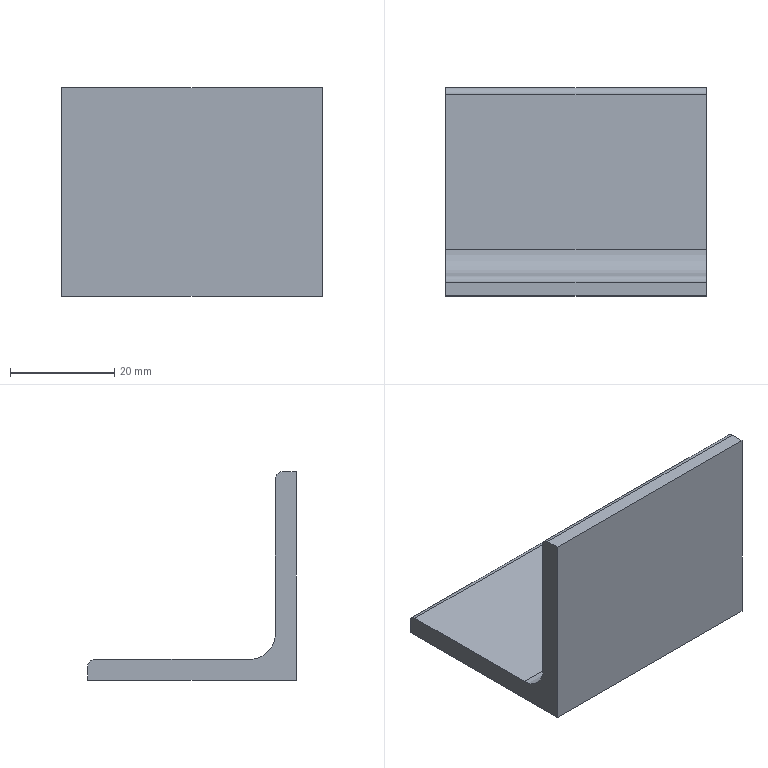Part | SolidWorks | features Extrusion 1 | 1 solid | 11 faces | box 50 x 40 x 40 mm | volume 15430 mm3 | plane 8 | cylinder 3 | commonest cylinder face diameters 2.667 x2 10 x1
STEP:
#1=CARTESIAN_POINT('',(0.,2.667,40.));
#2=VERTEX_POINT('',#1);
#3=CARTESIAN_POINT('',(0.,0.,40.));
#4=VERTEX_POINT('',#3);
#5=CARTESIAN_POINT('',(0.,0.,40.));
#6=DIRECTION('',(0.,-1.,0.));
#7=VECTOR('',#6,1000.);
#8=LINE('',#5,#7);
#9=EDGE_CURVE('',#2,#4,#8,.T.);
#10=ORIENTED_EDGE('',*,*,#9,.T.);
#11=CARTESIAN_POINT('',(50.,0.,40.));
#12=VERTEX_POINT('',#11);
#13=CARTESIAN_POINT('',(50.,0.,40.));
#14=DIRECTION('',(-1.,0.,0.));
#15=VECTOR('',#14,1000.);
#16=LINE('',#13,#15);
#17=EDGE_CURVE('',#12,#4,#16,.T.);
#18=ORIENTED_EDGE('',*,*,#17,.F.);
#19=CARTESIAN_POINT('',(50.,2.667,40.));
#20=VERTEX_POINT('',#19);
#21=CARTESIAN_POINT('',(50.,0.,40.));
#22=DIRECTION('',(0.,-1.,0.));
#23=VECTOR('',#22,1000.);
#24=LINE('',#21,#23);
#25=EDGE_CURVE('',#20,#12,#24,.T.);
#26=ORIENTED_EDGE('',*,*,#25,.F.);
#27=CARTESIAN_POINT('',(50.,2.667,40.));
#28=DIRECTION('',(-1.,0.,0.));
#29=VECTOR('',#28,1000.);
#30=LINE('',#27,#29);
#31=EDGE_CURVE('',#20,#2,#30,.T.);
#32=ORIENTED_EDGE('',*,*,#31,.T.);
#33=EDGE_LOOP('',(#10,#18,#26,#32));
#34=FACE_OUTER_BOUND('',#33,.T.);
#35=CARTESIAN_POINT('',(50.,0.,40.));
#36=DIRECTION('',(0.,0.,-1.));
#37=DIRECTION('',(0.,1.,0.));
#38=AXIS2_PLACEMENT_3D('',#35,#36,#37);
#39=PLANE('',#38);
#40=ADVANCED_FACE('',(#34),#39,.F.);
#41=CARTESIAN_POINT('',(0.,0.,0.));
#42=VERTEX_POINT('',#41);
#43=CARTESIAN_POINT('',(0.,0.,40.));
#44=DIRECTION('',(0.,0.,-1.));
#45=VECTOR('',#44,1000.);
#46=LINE('',#43,#45);
#47=EDGE_CURVE('',#4,#42,#46,.T.);
#48=ORIENTED_EDGE('',*,*,#47,.T.);
#49=CARTESIAN_POINT('',(50.,0.,0.));
#50=VERTEX_POINT('',#49);
#51=CARTESIAN_POINT('',(50.,0.,0.));
#52=DIRECTION('',(-1.,0.,0.));
#53=VECTOR('',#52,1000.);
#54=LINE('',#51,#53);
#55=EDGE_CURVE('',#50,#42,#54,.T.);
#56=ORIENTED_EDGE('',*,*,#55,.F.);
#57=CARTESIAN_POINT('',(50.,0.,40.));
#58=DIRECTION('',(0.,0.,-1.));
#59=VECTOR('',#58,1000.);
#60=LINE('',#57,#59);
#61=EDGE_CURVE('',#12,#50,#60,.T.);
#62=ORIENTED_EDGE('',*,*,#61,.F.);
#63=ORIENTED_EDGE('',*,*,#17,.T.);
#64=EDGE_LOOP('',(#48,#56,#62,#63));
#65=FACE_OUTER_BOUND('',#64,.T.);
#66=CARTESIAN_POINT('',(50.,0.,40.));
#67=DIRECTION('',(0.,1.,0.));
#68=DIRECTION('',(0.,0.,1.));
#69=AXIS2_PLACEMENT_3D('',#66,#67,#68);
#70=PLANE('',#69);
#71=ADVANCED_FACE('',(#65),#70,.F.);
#72=CARTESIAN_POINT('',(0.,40.,0.));
#73=VERTEX_POINT('',#72);
#74=CARTESIAN_POINT('',(0.,0.,0.));
#75=DIRECTION('',(0.,1.,0.));
#76=VECTOR('',#75,1000.);
#77=LINE('',#74,#76);
#78=EDGE_CURVE('',#42,#73,#77,.T.);
#79=ORIENTED_EDGE('',*,*,#78,.T.);
#80=CARTESIAN_POINT('',(50.,40.,0.));
#81=VERTEX_POINT('',#80);
#82=CARTESIAN_POINT('',(50.,40.,0.));
#83=DIRECTION('',(-1.,0.,0.));
#84=VECTOR('',#83,1000.);
#85=LINE('',#82,#84);
#86=EDGE_CURVE('',#81,#73,#85,.T.);
#87=ORIENTED_EDGE('',*,*,#86,.F.);
#88=CARTESIAN_POINT('',(50.,0.,0.));
#89=DIRECTION('',(0.,1.,0.));
#90=VECTOR('',#89,1000.);
#91=LINE('',#88,#90);
#92=EDGE_CURVE('',#50,#81,#91,.T.);
#93=ORIENTED_EDGE('',*,*,#92,.F.);
#94=ORIENTED_EDGE('',*,*,#55,.T.);
#95=EDGE_LOOP('',(#79,#87,#93,#94));
#96=FACE_OUTER_BOUND('',#95,.T.);
#97=CARTESIAN_POINT('',(50.,0.,0.));
#98=DIRECTION('',(0.,0.,1.));
#99=DIRECTION('',(1.,0.,0.));
#100=AXIS2_PLACEMENT_3D('',#97,#98,#99);
#101=PLANE('',#100);
#102=ADVANCED_FACE('',(#96),#101,.F.);
#103=CARTESIAN_POINT('',(0.,40.,2.667));
#104=VERTEX_POINT('',#103);
#105=CARTESIAN_POINT('',(0.,40.,0.));
#106=DIRECTION('',(0.,0.,1.));
#107=VECTOR('',#106,1000.);
#108=LINE('',#105,#107);
#109=EDGE_CURVE('',#73,#104,#108,.T.);
#110=ORIENTED_EDGE('',*,*,#109,.T.);
#111=CARTESIAN_POINT('',(50.,40.,2.667));
#112=VERTEX_POINT('',#111);
#113=CARTESIAN_POINT('',(50.,40.,2.667));
#114=DIRECTION('',(-1.,0.,0.));
#115=VECTOR('',#114,1000.);
#116=LINE('',#113,#115);
#117=EDGE_CURVE('',#112,#104,#116,.T.);
#118=ORIENTED_EDGE('',*,*,#117,.F.);
#119=CARTESIAN_POINT('',(50.,40.,0.));
#120=DIRECTION('',(0.,0.,1.));
#121=VECTOR('',#120,1000.);
#122=LINE('',#119,#121);
#123=EDGE_CURVE('',#81,#112,#122,.T.);
#124=ORIENTED_EDGE('',*,*,#123,.F.);
#125=ORIENTED_EDGE('',*,*,#86,.T.);
#126=EDGE_LOOP('',(#110,#118,#124,#125));
#127=FACE_OUTER_BOUND('',#126,.T.);
#128=CARTESIAN_POINT('',(50.,40.,0.));
#129=DIRECTION('',(0.,-1.,0.));
#130=DIRECTION('',(0.,0.,-1.));
#131=AXIS2_PLACEMENT_3D('',#128,#129,#130);
#132=PLANE('',#131);
#133=ADVANCED_FACE('',(#127),#132,.F.);
#134=CARTESIAN_POINT('',(0.,38.667,4.));
#135=VERTEX_POINT('',#134);
#136=CARTESIAN_POINT('',(0.,38.667,2.667));
#137=DIRECTION('',(1.,0.,0.));
#138=DIRECTION('',(0.,0.,-1.));
#139=AXIS2_PLACEMENT_3D('',#136,#137,#138);
#140=CIRCLE('',#139,1.333);
#141=EDGE_CURVE('',#104,#135,#140,.T.);
#142=ORIENTED_EDGE('',*,*,#141,.T.);
#143=CARTESIAN_POINT('',(50.,38.667,4.));
#144=VERTEX_POINT('',#143);
#145=CARTESIAN_POINT('',(50.,38.667,4.));
#146=DIRECTION('',(-1.,0.,0.));
#147=VECTOR('',#146,1000.);
#148=LINE('',#145,#147);
#149=EDGE_CURVE('',#144,#135,#148,.T.);
#150=ORIENTED_EDGE('',*,*,#149,.F.);
#151=CARTESIAN_POINT('',(50.,38.667,2.667));
#152=DIRECTION('',(1.,0.,0.));
#153=DIRECTION('',(0.,0.,-1.));
#154=AXIS2_PLACEMENT_3D('',#151,#152,#153);
#155=CIRCLE('',#154,1.333);
#156=EDGE_CURVE('',#112,#144,#155,.T.);
#157=ORIENTED_EDGE('',*,*,#156,.F.);
#158=ORIENTED_EDGE('',*,*,#117,.T.);
#159=EDGE_LOOP('',(#142,#150,#157,#158));
#160=FACE_OUTER_BOUND('',#159,.T.);
#161=CARTESIAN_POINT('',(50.,38.667,2.667));
#162=DIRECTION('',(-1.,0.,0.));
#163=DIRECTION('',(0.,0.,1.));
#164=AXIS2_PLACEMENT_3D('',#161,#162,#163);
#165=CYLINDRICAL_SURFACE('',#164,1.333);
#166=ADVANCED_FACE('',(#160),#165,.T.);
#167=CARTESIAN_POINT('',(0.,9.,4.));
#168=VERTEX_POINT('',#167);
#169=CARTESIAN_POINT('',(0.,9.,4.));
#170=DIRECTION('',(0.,-1.,0.));
#171=VECTOR('',#170,1000.);
#172=LINE('',#169,#171);
#173=EDGE_CURVE('',#135,#168,#172,.T.);
#174=ORIENTED_EDGE('',*,*,#173,.T.);
#175=CARTESIAN_POINT('',(50.,9.,4.));
#176=VERTEX_POINT('',#175);
#177=CARTESIAN_POINT('',(50.,9.,4.));
#178=DIRECTION('',(-1.,0.,0.));
#179=VECTOR('',#178,1000.);
#180=LINE('',#177,#179);
#181=EDGE_CURVE('',#176,#168,#180,.T.);
#182=ORIENTED_EDGE('',*,*,#181,.F.);
#183=CARTESIAN_POINT('',(50.,9.,4.));
#184=DIRECTION('',(0.,-1.,0.));
#185=VECTOR('',#184,1000.);
#186=LINE('',#183,#185);
#187=EDGE_CURVE('',#144,#176,#186,.T.);
#188=ORIENTED_EDGE('',*,*,#187,.F.);
#189=ORIENTED_EDGE('',*,*,#149,.T.);
#190=EDGE_LOOP('',(#174,#182,#188,#189));
#191=FACE_OUTER_BOUND('',#190,.T.);
#192=CARTESIAN_POINT('',(50.,9.,4.));
#193=DIRECTION('',(0.,0.,-1.));
#194=DIRECTION('',(-1.,0.,0.));
#195=AXIS2_PLACEMENT_3D('',#192,#193,#194);
#196=PLANE('',#195);
#197=ADVANCED_FACE('',(#191),#196,.F.);
#198=CARTESIAN_POINT('',(0.,4.,9.));
#199=VERTEX_POINT('',#198);
#200=CARTESIAN_POINT('',(0.,9.,9.));
#201=DIRECTION('',(-1.,0.,0.));
#202=DIRECTION('',(0.,0.,-1.));
#203=AXIS2_PLACEMENT_3D('',#200,#201,#202);
#204=CIRCLE('',#203,5.);
#205=EDGE_CURVE('',#168,#199,#204,.T.);
#206=ORIENTED_EDGE('',*,*,#205,.T.);
#207=CARTESIAN_POINT('',(50.,4.,9.));
#208=VERTEX_POINT('',#207);
#209=CARTESIAN_POINT('',(50.,4.,9.));
#210=DIRECTION('',(-1.,0.,0.));
#211=VECTOR('',#210,1000.);
#212=LINE('',#209,#211);
#213=EDGE_CURVE('',#208,#199,#212,.T.);
#214=ORIENTED_EDGE('',*,*,#213,.F.);
#215=CARTESIAN_POINT('',(50.,9.,9.));
#216=DIRECTION('',(-1.,0.,0.));
#217=DIRECTION('',(0.,0.,-1.));
#218=AXIS2_PLACEMENT_3D('',#215,#216,#217);
#219=CIRCLE('',#218,5.);
#220=EDGE_CURVE('',#176,#208,#219,.T.);
#221=ORIENTED_EDGE('',*,*,#220,.F.);
#222=ORIENTED_EDGE('',*,*,#181,.T.);
#223=EDGE_LOOP('',(#206,#214,#221,#222));
#224=FACE_OUTER_BOUND('',#223,.T.);
#225=CARTESIAN_POINT('',(50.,9.,9.));
#226=DIRECTION('',(-1.,0.,0.));
#227=DIRECTION('',(0.,0.,1.));
#228=AXIS2_PLACEMENT_3D('',#225,#226,#227);
#229=CYLINDRICAL_SURFACE('',#228,5.);
#230=ADVANCED_FACE('',(#224),#229,.F.);
#231=CARTESIAN_POINT('',(0.,4.,38.667));
#232=VERTEX_POINT('',#231);
#233=CARTESIAN_POINT('',(0.,4.,38.667));
#234=DIRECTION('',(0.,0.,1.));
#235=VECTOR('',#234,1000.);
#236=LINE('',#233,#235);
#237=EDGE_CURVE('',#199,#232,#236,.T.);
#238=ORIENTED_EDGE('',*,*,#237,.T.);
#239=CARTESIAN_POINT('',(50.,4.,38.667));
#240=VERTEX_POINT('',#239);
#241=CARTESIAN_POINT('',(50.,4.,38.667));
#242=DIRECTION('',(-1.,0.,0.));
#243=VECTOR('',#242,1000.);
#244=LINE('',#241,#243);
#245=EDGE_CURVE('',#240,#232,#244,.T.);
#246=ORIENTED_EDGE('',*,*,#245,.F.);
#247=CARTESIAN_POINT('',(50.,4.,38.667));
#248=DIRECTION('',(0.,0.,1.));
#249=VECTOR('',#248,1000.);
#250=LINE('',#247,#249);
#251=EDGE_CURVE('',#208,#240,#250,.T.);
#252=ORIENTED_EDGE('',*,*,#251,.F.);
#253=ORIENTED_EDGE('',*,*,#213,.T.);
#254=EDGE_LOOP('',(#238,#246,#252,#253));
#255=FACE_OUTER_BOUND('',#254,.T.);
#256=CARTESIAN_POINT('',(50.,4.,38.667));
#257=DIRECTION('',(0.,-1.,0.));
#258=DIRECTION('',(0.,0.,-1.));
#259=AXIS2_PLACEMENT_3D('',#256,#257,#258);
#260=PLANE('',#259);
#261=ADVANCED_FACE('',(#255),#260,.F.);
#262=CARTESIAN_POINT('',(0.,2.667,38.667));
#263=DIRECTION('',(1.,0.,0.));
#264=DIRECTION('',(0.,0.,1.));
#265=AXIS2_PLACEMENT_3D('',#262,#263,#264);
#266=CIRCLE('',#265,1.333);
#267=EDGE_CURVE('',#232,#2,#266,.T.);
#268=ORIENTED_EDGE('',*,*,#267,.T.);
#269=ORIENTED_EDGE('',*,*,#31,.F.);
#270=CARTESIAN_POINT('',(50.,2.667,38.667));
#271=DIRECTION('',(1.,0.,0.));
#272=DIRECTION('',(0.,0.,1.));
#273=AXIS2_PLACEMENT_3D('',#270,#271,#272);
#274=CIRCLE('',#273,1.333);
#275=EDGE_CURVE('',#240,#20,#274,.T.);
#276=ORIENTED_EDGE('',*,*,#275,.F.);
#277=ORIENTED_EDGE('',*,*,#245,.T.);
#278=EDGE_LOOP('',(#268,#269,#276,#277));
#279=FACE_OUTER_BOUND('',#278,.T.);
#280=CARTESIAN_POINT('',(50.,2.667,38.667));
#281=DIRECTION('',(-1.,0.,0.));
#282=DIRECTION('',(0.,0.,1.));
#283=AXIS2_PLACEMENT_3D('',#280,#281,#282);
#284=CYLINDRICAL_SURFACE('',#283,1.333);
#285=ADVANCED_FACE('',(#279),#284,.T.);
#286=ORIENTED_EDGE('',*,*,#25,.T.);
#287=ORIENTED_EDGE('',*,*,#61,.T.);
#288=ORIENTED_EDGE('',*,*,#92,.T.);
#289=ORIENTED_EDGE('',*,*,#123,.T.);
#290=ORIENTED_EDGE('',*,*,#156,.T.);
#291=ORIENTED_EDGE('',*,*,#187,.T.);
#292=ORIENTED_EDGE('',*,*,#220,.T.);
#293=ORIENTED_EDGE('',*,*,#251,.T.);
#294=ORIENTED_EDGE('',*,*,#275,.T.);
#295=EDGE_LOOP('',(#286,#287,#288,#289,#290,#291,#292,#293,#294));
#296=FACE_OUTER_BOUND('',#295,.T.);
#297=CARTESIAN_POINT('',(50.,2.667,38.667));
#298=DIRECTION('',(-1.,0.,0.));
#299=DIRECTION('',(0.,0.,1.));
#300=AXIS2_PLACEMENT_3D('',#297,#298,#299);
#301=PLANE('',#300);
#302=ADVANCED_FACE('',(#296),#301,.F.);
#303=ORIENTED_EDGE('',*,*,#9,.F.);
#304=ORIENTED_EDGE('',*,*,#267,.F.);
#305=ORIENTED_EDGE('',*,*,#237,.F.);
#306=ORIENTED_EDGE('',*,*,#205,.F.);
#307=ORIENTED_EDGE('',*,*,#173,.F.);
#308=ORIENTED_EDGE('',*,*,#141,.F.);
#309=ORIENTED_EDGE('',*,*,#109,.F.);
#310=ORIENTED_EDGE('',*,*,#78,.F.);
#311=ORIENTED_EDGE('',*,*,#47,.F.);
#312=EDGE_LOOP('',(#303,#304,#305,#306,#307,#308,#309,#310,#311));
#313=FACE_OUTER_BOUND('',#312,.T.);
#314=CARTESIAN_POINT('',(0.,2.667,38.667));
#315=DIRECTION('',(-1.,0.,0.));
#316=DIRECTION('',(0.,0.,1.));
#317=AXIS2_PLACEMENT_3D('',#314,#315,#316);
#318=PLANE('',#317);
#319=ADVANCED_FACE('',(#313),#318,.T.);
#320=CLOSED_SHELL('',(#40,#71,#102,#133,#166,#197,#230,#261,#285,#302,#319));
#321=MANIFOLD_SOLID_BREP('',#320);
#322=CARTESIAN_POINT('',(0.,0.,0.));
#323=DIRECTION('',(0.,0.,1.));
#324=DIRECTION('',(1.,0.,0.));
#325=AXIS2_PLACEMENT_3D('',#322,#323,#324);
#326=(LENGTH_UNIT()NAMED_UNIT(*)SI_UNIT(.MILLI.,.METRE.));
#327=UNCERTAINTY_MEASURE_WITH_UNIT(LENGTH_MEASURE(0.00001),#326,'','');
#328=(NAMED_UNIT(*)PLANE_ANGLE_UNIT()SI_UNIT($,.RADIAN.));
#329=(NAMED_UNIT(*)SI_UNIT($,.STERADIAN.)SOLID_ANGLE_UNIT());
#330=(GEOMETRIC_REPRESENTATION_CONTEXT(3)GLOBAL_UNCERTAINTY_ASSIGNED_CONTEXT((#327))GLOBAL_UNIT_ASSIGNED_CONTEXT((#326,#328,#329))REPRESENTATION_CONTEXT('',''));
#331=ADVANCED_BREP_SHAPE_REPRESENTATION('',(#321,#325),#330);